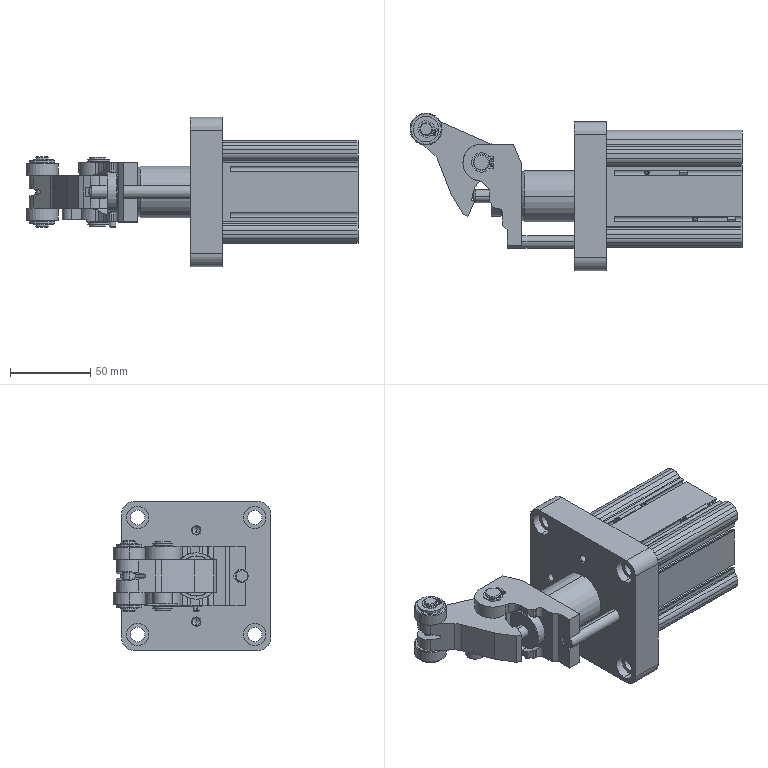Part | STEP file | 5 solids | 514 faces | box 207.005 x 98.34 x 93 mm | volume 532374 mm3 | cylinder 234 | plane 218 | cone 60 | spline 2 | commonest cylinder face diameters 8 x31 2 x29 14 x16 1 x13 4.34 x12 10 x12